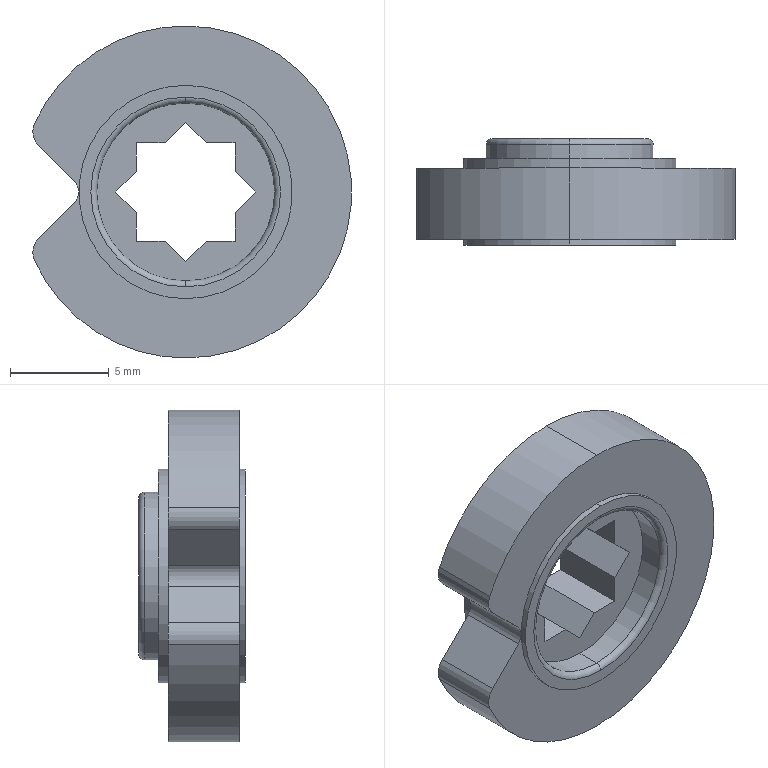Part | STEP file | PCS-04A-3_1_2.stp | 1 solid | 42 faces | box 16.138 x 5.4 x 16.8 mm | volume 681.99 mm3 | plane 24 | cylinder 14 | torus 4 | commonest cylinder face diameters 10.8 x4 16.8 x3 2 x2 8.5 x2 9 x2 1.568 x1
STEP:
#1=CARTESIAN_POINT('',(0.,5.1,3.95));
#2=VERTEX_POINT('',#1);
#3=CARTESIAN_POINT('',(0.,4.8,4.25));
#4=VERTEX_POINT('',#3);
#5=CARTESIAN_POINT('',(0.,4.8,3.95));
#6=DIRECTION('',(1.,0.,0.));
#7=DIRECTION('',(0.,1.,0.));
#8=AXIS2_PLACEMENT_3D('',#5,#6,#7);
#9=CIRCLE('',#8,0.3);
#10=EDGE_CURVE('',#2,#4,#9,.T.);
#11=ORIENTED_EDGE('',*,*,#10,.T.);
#12=CARTESIAN_POINT('',(0.,4.8,-4.25));
#13=VERTEX_POINT('',#12);
#14=CARTESIAN_POINT('',(0.,4.8,0.));
#15=DIRECTION('',(0.,-1.,0.));
#16=DIRECTION('',(0.,0.,-1.));
#17=AXIS2_PLACEMENT_3D('',#14,#15,#16);
#18=CIRCLE('',#17,4.25);
#19=EDGE_CURVE('',#13,#4,#18,.T.);
#20=ORIENTED_EDGE('',*,*,#19,.F.);
#21=CARTESIAN_POINT('',(0.,5.1,-3.95));
#22=VERTEX_POINT('',#21);
#23=CARTESIAN_POINT('',(0.,4.8,-3.95));
#24=DIRECTION('',(1.,0.,0.));
#25=DIRECTION('',(0.,0.,-1.));
#26=AXIS2_PLACEMENT_3D('',#23,#24,#25);
#27=CIRCLE('',#26,0.3);
#28=EDGE_CURVE('',#13,#22,#27,.T.);
#29=ORIENTED_EDGE('',*,*,#28,.T.);
#30=CARTESIAN_POINT('',(0.,5.1,0.));
#31=DIRECTION('',(0.,-1.,0.));
#32=DIRECTION('',(0.,0.,-1.));
#33=AXIS2_PLACEMENT_3D('',#30,#31,#32);
#34=CIRCLE('',#33,3.95);
#35=EDGE_CURVE('',#22,#2,#34,.T.);
#36=ORIENTED_EDGE('',*,*,#35,.T.);
#37=EDGE_LOOP('',(#11,#20,#29,#36));
#38=FACE_OUTER_BOUND('',#37,.T.);
#39=CARTESIAN_POINT('',(0.,4.8,0.));
#40=DIRECTION('',(0.,-1.,0.));
#41=DIRECTION('',(0.,0.,-1.));
#42=AXIS2_PLACEMENT_3D('',#39,#40,#41);
#43=TOROIDAL_SURFACE('',#42,3.95,0.3);
#44=ADVANCED_FACE('',(#38),#43,.T.);
#45=ORIENTED_EDGE('',*,*,#35,.F.);
#46=CARTESIAN_POINT('',(0.,5.1,0.));
#47=DIRECTION('',(0.,-1.,0.));
#48=DIRECTION('',(0.,0.,1.));
#49=AXIS2_PLACEMENT_3D('',#46,#47,#48);
#50=CIRCLE('',#49,3.95);
#51=EDGE_CURVE('',#2,#22,#50,.T.);
#52=ORIENTED_EDGE('',*,*,#51,.F.);
#53=EDGE_LOOP('',(#45,#52));
#54=FACE_OUTER_BOUND('',#53,.T.);
#55=CARTESIAN_POINT('',(-2.5,5.1,-2.5));
#56=VERTEX_POINT('',#55);
#57=CARTESIAN_POINT('',(-2.5,5.1,-1.036));
#58=VERTEX_POINT('',#57);
#59=CARTESIAN_POINT('',(-2.5,5.1,-2.5));
#60=DIRECTION('',(0.,0.,1.));
#61=VECTOR('',#60,1000.);
#62=LINE('',#59,#61);
#63=EDGE_CURVE('',#56,#58,#62,.T.);
#64=ORIENTED_EDGE('',*,*,#63,.F.);
#65=CARTESIAN_POINT('',(-1.036,5.1,-2.5));
#66=VERTEX_POINT('',#65);
#67=CARTESIAN_POINT('',(-1.036,5.1,-2.5));
#68=DIRECTION('',(-1.,0.,0.));
#69=VECTOR('',#68,1000.);
#70=LINE('',#67,#69);
#71=EDGE_CURVE('',#66,#56,#70,.T.);
#72=ORIENTED_EDGE('',*,*,#71,.F.);
#73=CARTESIAN_POINT('',(0.,5.1,-3.536));
#74=VERTEX_POINT('',#73);
#75=CARTESIAN_POINT('',(0.,5.1,-3.536));
#76=DIRECTION('',(-0.7071,0.,0.7071));
#77=VECTOR('',#76,1000.);
#78=LINE('',#75,#77);
#79=EDGE_CURVE('',#74,#66,#78,.T.);
#80=ORIENTED_EDGE('',*,*,#79,.F.);
#81=CARTESIAN_POINT('',(1.036,5.1,-2.5));
#82=VERTEX_POINT('',#81);
#83=CARTESIAN_POINT('',(0.,5.1,-3.536));
#84=DIRECTION('',(0.7071,0.,0.7071));
#85=VECTOR('',#84,1000.);
#86=LINE('',#83,#85);
#87=EDGE_CURVE('',#74,#82,#86,.T.);
#88=ORIENTED_EDGE('',*,*,#87,.T.);
#89=CARTESIAN_POINT('',(2.5,5.1,-2.5));
#90=VERTEX_POINT('',#89);
#91=CARTESIAN_POINT('',(2.5,5.1,-2.5));
#92=DIRECTION('',(-1.,0.,0.));
#93=VECTOR('',#92,1000.);
#94=LINE('',#91,#93);
#95=EDGE_CURVE('',#90,#82,#94,.T.);
#96=ORIENTED_EDGE('',*,*,#95,.F.);
#97=CARTESIAN_POINT('',(2.5,5.1,-1.036));
#98=VERTEX_POINT('',#97);
#99=CARTESIAN_POINT('',(2.5,5.1,-1.036));
#100=DIRECTION('',(0.,0.,-1.));
#101=VECTOR('',#100,1000.);
#102=LINE('',#99,#101);
#103=EDGE_CURVE('',#98,#90,#102,.T.);
#104=ORIENTED_EDGE('',*,*,#103,.F.);
#105=CARTESIAN_POINT('',(3.536,5.1,0.));
#106=VERTEX_POINT('',#105);
#107=CARTESIAN_POINT('',(2.5,5.1,-1.036));
#108=DIRECTION('',(0.7071,0.,0.7071));
#109=VECTOR('',#108,1000.);
#110=LINE('',#107,#109);
#111=EDGE_CURVE('',#98,#106,#110,.T.);
#112=ORIENTED_EDGE('',*,*,#111,.T.);
#113=CARTESIAN_POINT('',(2.5,5.1,1.036));
#114=VERTEX_POINT('',#113);
#115=CARTESIAN_POINT('',(2.5,5.1,1.036));
#116=DIRECTION('',(0.7071,0.,-0.7071));
#117=VECTOR('',#116,1000.);
#118=LINE('',#115,#117);
#119=EDGE_CURVE('',#114,#106,#118,.T.);
#120=ORIENTED_EDGE('',*,*,#119,.F.);
#121=CARTESIAN_POINT('',(2.5,5.1,2.5));
#122=VERTEX_POINT('',#121);
#123=CARTESIAN_POINT('',(2.5,5.1,2.5));
#124=DIRECTION('',(0.,0.,-1.));
#125=VECTOR('',#124,1000.);
#126=LINE('',#123,#125);
#127=EDGE_CURVE('',#122,#114,#126,.T.);
#128=ORIENTED_EDGE('',*,*,#127,.F.);
#129=CARTESIAN_POINT('',(1.036,5.1,2.5));
#130=VERTEX_POINT('',#129);
#131=CARTESIAN_POINT('',(1.036,5.1,2.5));
#132=DIRECTION('',(1.,0.,0.));
#133=VECTOR('',#132,1000.);
#134=LINE('',#131,#133);
#135=EDGE_CURVE('',#130,#122,#134,.T.);
#136=ORIENTED_EDGE('',*,*,#135,.F.);
#137=CARTESIAN_POINT('',(0.,5.1,3.536));
#138=VERTEX_POINT('',#137);
#139=CARTESIAN_POINT('',(0.,5.1,3.536));
#140=DIRECTION('',(0.7071,0.,-0.7071));
#141=VECTOR('',#140,1000.);
#142=LINE('',#139,#141);
#143=EDGE_CURVE('',#138,#130,#142,.T.);
#144=ORIENTED_EDGE('',*,*,#143,.F.);
#145=CARTESIAN_POINT('',(-1.036,5.1,2.5));
#146=VERTEX_POINT('',#145);
#147=CARTESIAN_POINT('',(0.,5.1,3.536));
#148=DIRECTION('',(-0.7071,0.,-0.7071));
#149=VECTOR('',#148,1000.);
#150=LINE('',#147,#149);
#151=EDGE_CURVE('',#138,#146,#150,.T.);
#152=ORIENTED_EDGE('',*,*,#151,.T.);
#153=CARTESIAN_POINT('',(-2.5,5.1,2.5));
#154=VERTEX_POINT('',#153);
#155=CARTESIAN_POINT('',(-2.5,5.1,2.5));
#156=DIRECTION('',(1.,0.,0.));
#157=VECTOR('',#156,1000.);
#158=LINE('',#155,#157);
#159=EDGE_CURVE('',#154,#146,#158,.T.);
#160=ORIENTED_EDGE('',*,*,#159,.F.);
#161=CARTESIAN_POINT('',(-2.5,5.1,1.036));
#162=VERTEX_POINT('',#161);
#163=CARTESIAN_POINT('',(-2.5,5.1,1.036));
#164=DIRECTION('',(0.,0.,1.));
#165=VECTOR('',#164,1000.);
#166=LINE('',#163,#165);
#167=EDGE_CURVE('',#162,#154,#166,.T.);
#168=ORIENTED_EDGE('',*,*,#167,.F.);
#169=CARTESIAN_POINT('',(-3.536,5.1,0.));
#170=VERTEX_POINT('',#169);
#171=CARTESIAN_POINT('',(-2.5,5.1,1.036));
#172=DIRECTION('',(-0.7071,0.,-0.7071));
#173=VECTOR('',#172,1000.);
#174=LINE('',#171,#173);
#175=EDGE_CURVE('',#162,#170,#174,.T.);
#176=ORIENTED_EDGE('',*,*,#175,.T.);
#177=CARTESIAN_POINT('',(-2.5,5.1,-1.036));
#178=DIRECTION('',(-0.7071,0.,0.7071));
#179=VECTOR('',#178,1000.);
#180=LINE('',#177,#179);
#181=EDGE_CURVE('',#58,#170,#180,.T.);
#182=ORIENTED_EDGE('',*,*,#181,.F.);
#183=EDGE_LOOP('',(#64,#72,#80,#88,#96,#104,#112,#120,#128,#136,#144,#152,#160,#168,#176,#182));
#184=FACE_BOUND('',#183,.T.);
#185=CARTESIAN_POINT('',(0.,5.1,0.));
#186=DIRECTION('',(0.,-1.,0.));
#187=DIRECTION('',(0.,0.,-1.));
#188=AXIS2_PLACEMENT_3D('',#185,#186,#187);
#189=PLANE('',#188);
#190=ADVANCED_FACE('',(#54,#184),#189,.F.);
#191=ORIENTED_EDGE('',*,*,#51,.T.);
#192=ORIENTED_EDGE('',*,*,#28,.F.);
#193=CARTESIAN_POINT('',(0.,4.8,0.));
#194=DIRECTION('',(0.,-1.,0.));
#195=DIRECTION('',(0.,0.,1.));
#196=AXIS2_PLACEMENT_3D('',#193,#194,#195);
#197=CIRCLE('',#196,4.25);
#198=EDGE_CURVE('',#4,#13,#197,.T.);
#199=ORIENTED_EDGE('',*,*,#198,.F.);
#200=ORIENTED_EDGE('',*,*,#10,.F.);
#201=EDGE_LOOP('',(#191,#192,#199,#200));
#202=FACE_OUTER_BOUND('',#201,.T.);
#203=CARTESIAN_POINT('',(0.,4.8,0.));
#204=DIRECTION('',(0.,-1.,0.));
#205=DIRECTION('',(0.,0.,-1.));
#206=AXIS2_PLACEMENT_3D('',#203,#204,#205);
#207=TOROIDAL_SURFACE('',#206,3.95,0.3);
#208=ADVANCED_FACE('',(#202),#207,.T.);
#209=ORIENTED_EDGE('',*,*,#198,.T.);
#210=CARTESIAN_POINT('',(0.,4.1,-4.25));
#211=VERTEX_POINT('',#210);
#212=CARTESIAN_POINT('',(0.,4.1,-4.25));
#213=DIRECTION('',(0.,1.,0.));
#214=VECTOR('',#213,1000.);
#215=LINE('',#212,#214);
#216=EDGE_CURVE('',#211,#13,#215,.T.);
#217=ORIENTED_EDGE('',*,*,#216,.F.);
#218=CARTESIAN_POINT('',(0.,4.1,4.25));
#219=VERTEX_POINT('',#218);
#220=CARTESIAN_POINT('',(0.,4.1,0.));
#221=DIRECTION('',(0.,1.,0.));
#222=DIRECTION('',(0.,0.,-1.));
#223=AXIS2_PLACEMENT_3D('',#220,#221,#222);
#224=CIRCLE('',#223,4.25);
#225=EDGE_CURVE('',#211,#219,#224,.T.);
#226=ORIENTED_EDGE('',*,*,#225,.T.);
#227=CARTESIAN_POINT('',(0.,4.8,4.25));
#228=DIRECTION('',(0.,-1.,0.));
#229=VECTOR('',#228,1000.);
#230=LINE('',#227,#229);
#231=EDGE_CURVE('',#4,#219,#230,.T.);
#232=ORIENTED_EDGE('',*,*,#231,.F.);
#233=EDGE_LOOP('',(#209,#217,#226,#232));
#234=FACE_OUTER_BOUND('',#233,.T.);
#235=CARTESIAN_POINT('',(0.,4.1,0.));
#236=DIRECTION('',(0.,-1.,0.));
#237=DIRECTION('',(0.,0.,-1.));
#238=AXIS2_PLACEMENT_3D('',#235,#236,#237);
#239=CYLINDRICAL_SURFACE('',#238,4.25);
#240=ADVANCED_FACE('',(#234),#239,.T.);
#241=ORIENTED_EDGE('',*,*,#231,.T.);
#242=CARTESIAN_POINT('',(0.,4.1,0.));
#243=DIRECTION('',(0.,1.,0.));
#244=DIRECTION('',(0.,0.,1.));
#245=AXIS2_PLACEMENT_3D('',#242,#243,#244);
#246=CIRCLE('',#245,4.25);
#247=EDGE_CURVE('',#219,#211,#246,.T.);
#248=ORIENTED_EDGE('',*,*,#247,.T.);
#249=ORIENTED_EDGE('',*,*,#216,.T.);
#250=ORIENTED_EDGE('',*,*,#19,.T.);
#251=EDGE_LOOP('',(#241,#248,#249,#250));
#252=FACE_OUTER_BOUND('',#251,.T.);
#253=CARTESIAN_POINT('',(0.,4.1,0.));
#254=DIRECTION('',(0.,-1.,0.));
#255=DIRECTION('',(0.,0.,-1.));
#256=AXIS2_PLACEMENT_3D('',#253,#254,#255);
#257=CYLINDRICAL_SURFACE('',#256,4.25);
#258=ADVANCED_FACE('',(#252),#257,.T.);
#259=CARTESIAN_POINT('',(0.,4.1,-5.4));
#260=VERTEX_POINT('',#259);
#261=CARTESIAN_POINT('',(0.,4.1,5.4));
#262=VERTEX_POINT('',#261);
#263=CARTESIAN_POINT('',(0.,4.1,0.));
#264=DIRECTION('',(0.,-1.,0.));
#265=DIRECTION('',(0.,0.,-1.));
#266=AXIS2_PLACEMENT_3D('',#263,#264,#265);
#267=CIRCLE('',#266,5.4);
#268=EDGE_CURVE('',#260,#262,#267,.T.);
#269=ORIENTED_EDGE('',*,*,#268,.F.);
#270=CARTESIAN_POINT('',(0.,4.1,0.));
#271=DIRECTION('',(0.,-1.,0.));
#272=DIRECTION('',(0.,0.,1.));
#273=AXIS2_PLACEMENT_3D('',#270,#271,#272);
#274=CIRCLE('',#273,5.4);
#275=EDGE_CURVE('',#262,#260,#274,.T.);
#276=ORIENTED_EDGE('',*,*,#275,.F.);
#277=EDGE_LOOP('',(#269,#276));
#278=FACE_OUTER_BOUND('',#277,.T.);
#279=ORIENTED_EDGE('',*,*,#247,.F.);
#280=ORIENTED_EDGE('',*,*,#225,.F.);
#281=EDGE_LOOP('',(#279,#280));
#282=FACE_BOUND('',#281,.T.);
#283=CARTESIAN_POINT('',(0.,4.1,0.));
#284=DIRECTION('',(0.,1.,0.));
#285=DIRECTION('',(1.,0.,0.));
#286=AXIS2_PLACEMENT_3D('',#283,#284,#285);
#287=PLANE('',#286);
#288=ADVANCED_FACE('',(#278,#282),#287,.T.);
#289=ORIENTED_EDGE('',*,*,#275,.T.);
#290=CARTESIAN_POINT('',(0.,3.6,-5.4));
#291=VERTEX_POINT('',#290);
#292=CARTESIAN_POINT('',(0.,3.6,-5.4));
#293=DIRECTION('',(0.,1.,0.));
#294=VECTOR('',#293,1000.);
#295=LINE('',#292,#294);
#296=EDGE_CURVE('',#291,#260,#295,.T.);
#297=ORIENTED_EDGE('',*,*,#296,.F.);
#298=CARTESIAN_POINT('',(0.,3.6,5.4));
#299=VERTEX_POINT('',#298);
#300=CARTESIAN_POINT('',(0.,3.6,0.));
#301=DIRECTION('',(0.,1.,0.));
#302=DIRECTION('',(0.,0.,-1.));
#303=AXIS2_PLACEMENT_3D('',#300,#301,#302);
#304=CIRCLE('',#303,5.4);
#305=EDGE_CURVE('',#291,#299,#304,.T.);
#306=ORIENTED_EDGE('',*,*,#305,.T.);
#307=CARTESIAN_POINT('',(0.,4.1,5.4));
#308=DIRECTION('',(0.,-1.,0.));
#309=VECTOR('',#308,1000.);
#310=LINE('',#307,#309);
#311=EDGE_CURVE('',#262,#299,#310,.T.);
#312=ORIENTED_EDGE('',*,*,#311,.F.);
#313=EDGE_LOOP('',(#289,#297,#306,#312));
#314=FACE_OUTER_BOUND('',#313,.T.);
#315=CARTESIAN_POINT('',(0.,3.6,0.));
#316=DIRECTION('',(0.,-1.,0.));
#317=DIRECTION('',(0.,0.,-1.));
#318=AXIS2_PLACEMENT_3D('',#315,#316,#317);
#319=CYLINDRICAL_SURFACE('',#318,5.4);
#320=ADVANCED_FACE('',(#314),#319,.T.);
#321=ORIENTED_EDGE('',*,*,#311,.T.);
#322=CARTESIAN_POINT('',(0.,3.6,0.));
#323=DIRECTION('',(0.,1.,0.));
#324=DIRECTION('',(0.,0.,1.));
#325=AXIS2_PLACEMENT_3D('',#322,#323,#324);
#326=CIRCLE('',#325,5.4);
#327=EDGE_CURVE('',#299,#291,#326,.T.);
#328=ORIENTED_EDGE('',*,*,#327,.T.);
#329=ORIENTED_EDGE('',*,*,#296,.T.);
#330=ORIENTED_EDGE('',*,*,#268,.T.);
#331=EDGE_LOOP('',(#321,#328,#329,#330));
#332=FACE_OUTER_BOUND('',#331,.T.);
#333=CARTESIAN_POINT('',(0.,3.6,0.));
#334=DIRECTION('',(0.,-1.,0.));
#335=DIRECTION('',(0.,0.,-1.));
#336=AXIS2_PLACEMENT_3D('',#333,#334,#335);
#337=CYLINDRICAL_SURFACE('',#336,5.4);
#338=ADVANCED_FACE('',(#332),#337,.T.);
#339=CARTESIAN_POINT('',(0.,3.6,-8.4));
#340=VERTEX_POINT('',#339);
#341=CARTESIAN_POINT('',(0.,3.6,8.4));
#342=VERTEX_POINT('',#341);
#343=CARTESIAN_POINT('',(0.,3.6,0.));
#344=DIRECTION('',(0.,-1.,0.));
#345=DIRECTION('',(0.,0.,-1.));
#346=AXIS2_PLACEMENT_3D('',#343,#344,#345);
#347=CIRCLE('',#346,8.4);
#348=EDGE_CURVE('',#340,#342,#347,.T.);
#349=ORIENTED_EDGE('',*,*,#348,.F.);
#350=CARTESIAN_POINT('',(-7.649,3.6,-3.472));
#351=VERTEX_POINT('',#350);
#352=CARTESIAN_POINT('',(0.,3.6,0.));
#353=DIRECTION('',(0.,-1.,0.));
#354=DIRECTION('',(-0.9106,0.,-0.4133));
#355=AXIS2_PLACEMENT_3D('',#352,#353,#354);
#356=CIRCLE('',#355,8.4);
#357=EDGE_CURVE('',#351,#340,#356,.T.);
#358=ORIENTED_EDGE('',*,*,#357,.F.);
#359=CARTESIAN_POINT('',(-7.446,3.6,-2.351));
#360=VERTEX_POINT('',#359);
#361=CARTESIAN_POINT('',(-6.738,3.6,-3.058));
#362=DIRECTION('',(0.,-1.,0.));
#363=DIRECTION('',(-0.7071,0.,0.7071));
#364=AXIS2_PLACEMENT_3D('',#361,#362,#363);
#365=CIRCLE('',#364,1.);
#366=EDGE_CURVE('',#360,#351,#365,.T.);
#367=ORIENTED_EDGE('',*,*,#366,.F.);
#368=CARTESIAN_POINT('',(-5.607,3.6,-0.5127));
#369=VERTEX_POINT('',#368);
#370=CARTESIAN_POINT('',(-7.446,3.6,-2.351));
#371=DIRECTION('',(0.7071,0.,0.7071));
#372=VECTOR('',#371,1000.);
#373=LINE('',#370,#372);
#374=EDGE_CURVE('',#360,#369,#373,.T.);
#375=ORIENTED_EDGE('',*,*,#374,.T.);
#376=CARTESIAN_POINT('',(-5.607,3.6,0.5127));
#377=VERTEX_POINT('',#376);
#378=CARTESIAN_POINT('',(-6.2,3.6,0.));
#379=DIRECTION('',(0.,1.,0.));
#380=DIRECTION('',(0.7564,0.,0.6541));
#381=AXIS2_PLACEMENT_3D('',#378,#379,#380);
#382=CIRCLE('',#381,0.7838);
#383=EDGE_CURVE('',#377,#369,#382,.T.);
#384=ORIENTED_EDGE('',*,*,#383,.F.);
#385=CARTESIAN_POINT('',(-7.446,3.6,2.351));
#386=VERTEX_POINT('',#385);
#387=CARTESIAN_POINT('',(-5.607,3.6,0.5127));
#388=DIRECTION('',(-0.7071,0.,0.7071));
#389=VECTOR('',#388,1000.);
#390=LINE('',#387,#389);
#391=EDGE_CURVE('',#377,#386,#390,.T.);
#392=ORIENTED_EDGE('',*,*,#391,.T.);
#393=CARTESIAN_POINT('',(-7.649,3.6,3.472));
#394=VERTEX_POINT('',#393);
#395=CARTESIAN_POINT('',(-6.738,3.6,3.058));
#396=DIRECTION('',(0.,-1.,0.));
#397=DIRECTION('',(-0.9106,0.,0.4133));
#398=AXIS2_PLACEMENT_3D('',#395,#396,#397);
#399=CIRCLE('',#398,1.);
#400=EDGE_CURVE('',#394,#386,#399,.T.);
#401=ORIENTED_EDGE('',*,*,#400,.F.);
#402=CARTESIAN_POINT('',(0.,3.6,0.));
#403=DIRECTION('',(0.,-1.,0.));
#404=DIRECTION('',(0.,0.,1.));
#405=AXIS2_PLACEMENT_3D('',#402,#403,#404);
#406=CIRCLE('',#405,8.4);
#407=EDGE_CURVE('',#342,#394,#406,.T.);
#408=ORIENTED_EDGE('',*,*,#407,.F.);
#409=EDGE_LOOP('',(#349,#358,#367,#375,#384,#392,#401,#408));
#410=FACE_OUTER_BOUND('',#409,.T.);
#411=ORIENTED_EDGE('',*,*,#327,.F.);
#412=ORIENTED_EDGE('',*,*,#305,.F.);
#413=EDGE_LOOP('',(#411,#412));
#414=FACE_BOUND('',#413,.T.);
#415=CARTESIAN_POINT('',(0.,3.6,0.));
#416=DIRECTION('',(0.,1.,0.));
#417=DIRECTION('',(1.,0.,0.));
#418=AXIS2_PLACEMENT_3D('',#415,#416,#417);
#419=PLANE('',#418);
#420=ADVANCED_FACE('',(#410,#414),#419,.T.);
#421=ORIENTED_EDGE('',*,*,#407,.T.);
#422=CARTESIAN_POINT('',(-7.649,0.,3.472));
#423=VERTEX_POINT('',#422);
#424=CARTESIAN_POINT('',(-7.649,3.6,3.472));
#425=DIRECTION('',(0.,-1.,0.));
#426=VECTOR('',#425,1000.);
#427=LINE('',#424,#426);
#428=EDGE_CURVE('',#394,#423,#427,.T.);
#429=ORIENTED_EDGE('',*,*,#428,.T.);
#430=CARTESIAN_POINT('',(0.,0.,8.4));
#431=VERTEX_POINT('',#430);
#432=CARTESIAN_POINT('',(0.,0.,0.));
#433=DIRECTION('',(0.,1.,0.));
#434=DIRECTION('',(-0.9106,0.,0.4133));
#435=AXIS2_PLACEMENT_3D('',#432,#433,#434);
#436=CIRCLE('',#435,8.4);
#437=EDGE_CURVE('',#423,#431,#436,.T.);
#438=ORIENTED_EDGE('',*,*,#437,.T.);
#439=CARTESIAN_POINT('',(0.,3.6,8.4));
#440=DIRECTION('',(0.,-1.,0.));
#441=VECTOR('',#440,1000.);
#442=LINE('',#439,#441);
#443=EDGE_CURVE('',#342,#431,#442,.T.);
#444=ORIENTED_EDGE('',*,*,#443,.F.);
#445=EDGE_LOOP('',(#421,#429,#438,#444));
#446=FACE_OUTER_BOUND('',#445,.T.);
#447=CARTESIAN_POINT('',(0.,0.,0.));
#448=DIRECTION('',(0.,-1.,0.));
#449=DIRECTION('',(0.,0.,-1.));
#450=AXIS2_PLACEMENT_3D('',#447,#448,#449);
#451=CYLINDRICAL_SURFACE('',#450,8.4);
#452=ADVANCED_FACE('',(#446),#451,.T.);
#453=ORIENTED_EDGE('',*,*,#443,.T.);
#454=CARTESIAN_POINT('',(0.,0.,-8.4));
#455=VERTEX_POINT('',#454);
#456=CARTESIAN_POINT('',(0.,0.,0.));
#457=DIRECTION('',(0.,1.,0.));
#458=DIRECTION('',(0.,0.,1.));
#459=AXIS2_PLACEMENT_3D('',#456,#457,#458);
#460=CIRCLE('',#459,8.4);
#461=EDGE_CURVE('',#431,#455,#460,.T.);
#462=ORIENTED_EDGE('',*,*,#461,.T.);
#463=CARTESIAN_POINT('',(0.,0.,-8.4));
#464=DIRECTION('',(0.,1.,0.));
#465=VECTOR('',#464,1000.);
#466=LINE('',#463,#465);
#467=EDGE_CURVE('',#455,#340,#466,.T.);
#468=ORIENTED_EDGE('',*,*,#467,.T.);
#469=ORIENTED_EDGE('',*,*,#348,.T.);
#470=EDGE_LOOP('',(#453,#462,#468,#469));
#471=FACE_OUTER_BOUND('',#470,.T.);
#472=CARTESIAN_POINT('',(0.,0.,0.));
#473=DIRECTION('',(0.,-1.,0.));
#474=DIRECTION('',(0.,0.,-1.));
#475=AXIS2_PLACEMENT_3D('',#472,#473,#474);
#476=CYLINDRICAL_SURFACE('',#475,8.4);
#477=ADVANCED_FACE('',(#471),#476,.T.);
#478=ORIENTED_EDGE('',*,*,#467,.F.);
#479=CARTESIAN_POINT('',(-7.649,0.,-3.472));
#480=VERTEX_POINT('',#479);
#481=CARTESIAN_POINT('',(0.,0.,0.));
#482=DIRECTION('',(0.,1.,0.));
#483=DIRECTION('',(0.,0.,-1.));
#484=AXIS2_PLACEMENT_3D('',#481,#482,#483);
#485=CIRCLE('',#484,8.4);
#486=EDGE_CURVE('',#455,#480,#485,.T.);
#487=ORIENTED_EDGE('',*,*,#486,.T.);
#488=CARTESIAN_POINT('',(-7.649,0.,-3.472));
#489=DIRECTION('',(0.,1.,0.));
#490=VECTOR('',#489,1000.);
#491=LINE('',#488,#490);
#492=EDGE_CURVE('',#480,#351,#491,.T.);
#493=ORIENTED_EDGE('',*,*,#492,.T.);
#494=ORIENTED_EDGE('',*,*,#357,.T.);
#495=EDGE_LOOP('',(#478,#487,#493,#494));
#496=FACE_OUTER_BOUND('',#495,.T.);
#497=CARTESIAN_POINT('',(0.,0.,0.));
#498=DIRECTION('',(0.,-1.,0.));
#499=DIRECTION('',(0.,0.,-1.));
#500=AXIS2_PLACEMENT_3D('',#497,#498,#499);
#501=CYLINDRICAL_SURFACE('',#500,8.4);
#502=ADVANCED_FACE('',(#496),#501,.T.);
#503=ORIENTED_EDGE('',*,*,#492,.F.);
#504=CARTESIAN_POINT('',(-7.446,0.,-2.351));
#505=VERTEX_POINT('',#504);
#506=CARTESIAN_POINT('',(-6.738,0.,-3.058));
#507=DIRECTION('',(0.,1.,0.));
#508=DIRECTION('',(-0.9106,0.,-0.4133));
#509=AXIS2_PLACEMENT_3D('',#506,#507,#508);
#510=CIRCLE('',#509,1.);
#511=EDGE_CURVE('',#480,#505,#510,.T.);
#512=ORIENTED_EDGE('',*,*,#511,.T.);
#513=CARTESIAN_POINT('',(-7.446,0.,-2.351));
#514=DIRECTION('',(0.,1.,0.));
#515=VECTOR('',#514,1000.);
#516=LINE('',#513,#515);
#517=EDGE_CURVE('',#505,#360,#516,.T.);
#518=ORIENTED_EDGE('',*,*,#517,.T.);
#519=ORIENTED_EDGE('',*,*,#366,.T.);
#520=EDGE_LOOP('',(#503,#512,#518,#519));
#521=FACE_OUTER_BOUND('',#520,.T.);
#522=CARTESIAN_POINT('',(-6.738,3.6,-3.058));
#523=DIRECTION('',(0.,1.,0.));
#524=DIRECTION('',(0.,0.,1.));
#525=AXIS2_PLACEMENT_3D('',#522,#523,#524);
#526=CYLINDRICAL_SURFACE('',#525,1.);
#527=ADVANCED_FACE('',(#521),#526,.T.);
#528=ORIENTED_EDGE('',*,*,#517,.F.);
#529=CARTESIAN_POINT('',(-5.607,0.,-0.5127));
#530=VERTEX_POINT('',#529);
#531=CARTESIAN_POINT('',(-5.607,0.,-0.5127));
#532=DIRECTION('',(-0.7071,0.,-0.7071));
#533=VECTOR('',#532,1000.);
#534=LINE('',#531,#533);
#535=EDGE_CURVE('',#530,#505,#534,.T.);
#536=ORIENTED_EDGE('',*,*,#535,.F.);
#537=CARTESIAN_POINT('',(-5.607,3.6,-0.5127));
#538=DIRECTION('',(0.,-1.,0.));
#539=VECTOR('',#538,1000.);
#540=LINE('',#537,#539);
#541=EDGE_CURVE('',#369,#530,#540,.T.);
#542=ORIENTED_EDGE('',*,*,#541,.F.);
#543=ORIENTED_EDGE('',*,*,#374,.F.);
#544=EDGE_LOOP('',(#528,#536,#542,#543));
#545=FACE_OUTER_BOUND('',#544,.T.);
#546=CARTESIAN_POINT('',(-11.858,0.,-6.764));
#547=DIRECTION('',(0.7071,0.,-0.7071));
#548=DIRECTION('',(0.,-1.,0.));
#549=AXIS2_PLACEMENT_3D('',#546,#547,#548);
#550=PLANE('',#549);
#551=ADVANCED_FACE('',(#545),#550,.F.);
#552=ORIENTED_EDGE('',*,*,#541,.T.);
#553=CARTESIAN_POINT('',(-5.607,0.,0.5127));
#554=VERTEX_POINT('',#553);
#555=CARTESIAN_POINT('',(-6.2,0.,0.));
#556=DIRECTION('',(0.,-1.,0.));
#557=DIRECTION('',(0.7564,0.,-0.6541));
#558=AXIS2_PLACEMENT_3D('',#555,#556,#557);
#559=CIRCLE('',#558,0.7838);
#560=EDGE_CURVE('',#530,#554,#559,.T.);
#561=ORIENTED_EDGE('',*,*,#560,.T.);
#562=CARTESIAN_POINT('',(-5.607,3.6,0.5127));
#563=DIRECTION('',(0.,-1.,0.));
#564=VECTOR('',#563,1000.);
#565=LINE('',#562,#564);
#566=EDGE_CURVE('',#377,#554,#565,.T.);
#567=ORIENTED_EDGE('',*,*,#566,.F.);
#568=ORIENTED_EDGE('',*,*,#383,.T.);
#569=EDGE_LOOP('',(#552,#561,#567,#568));
#570=FACE_OUTER_BOUND('',#569,.T.);
#571=CARTESIAN_POINT('',(-6.2,0.,0.));
#572=DIRECTION('',(0.,1.,0.));
#573=DIRECTION('',(0.,0.,1.));
#574=AXIS2_PLACEMENT_3D('',#571,#572,#573);
#575=CYLINDRICAL_SURFACE('',#574,0.7838);
#576=ADVANCED_FACE('',(#570),#575,.F.);
#577=ORIENTED_EDGE('',*,*,#566,.T.);
#578=CARTESIAN_POINT('',(-7.446,0.,2.351));
#579=VERTEX_POINT('',#578);
#580=CARTESIAN_POINT('',(-7.446,0.,2.351));
#581=DIRECTION('',(0.7071,0.,-0.7071));
#582=VECTOR('',#581,1000.);
#583=LINE('',#580,#582);
#584=EDGE_CURVE('',#579,#554,#583,.T.);
#585=ORIENTED_EDGE('',*,*,#584,.F.);
#586=CARTESIAN_POINT('',(-7.446,0.,2.351));
#587=DIRECTION('',(0.,1.,0.));
#588=VECTOR('',#587,1000.);
#589=LINE('',#586,#588);
#590=EDGE_CURVE('',#579,#386,#589,.T.);
#591=ORIENTED_EDGE('',*,*,#590,.T.);
#592=ORIENTED_EDGE('',*,*,#391,.F.);
#593=EDGE_LOOP('',(#577,#585,#591,#592));
#594=FACE_OUTER_BOUND('',#593,.T.);
#595=CARTESIAN_POINT('',(-11.858,0.,6.764));
#596=DIRECTION('',(-0.7071,0.,-0.7071));
#597=DIRECTION('',(-0.7071,0.,0.7071));
#598=AXIS2_PLACEMENT_3D('',#595,#596,#597);
#599=PLANE('',#598);
#600=ADVANCED_FACE('',(#594),#599,.T.);
#601=ORIENTED_EDGE('',*,*,#590,.F.);
#602=CARTESIAN_POINT('',(-6.738,0.,3.058));
#603=DIRECTION('',(0.,1.,0.));
#604=DIRECTION('',(-0.7071,0.,-0.7071));
#605=AXIS2_PLACEMENT_3D('',#602,#603,#604);
#606=CIRCLE('',#605,1.);
#607=EDGE_CURVE('',#579,#423,#606,.T.);
#608=ORIENTED_EDGE('',*,*,#607,.T.);
#609=ORIENTED_EDGE('',*,*,#428,.F.);
#610=ORIENTED_EDGE('',*,*,#400,.T.);
#611=EDGE_LOOP('',(#601,#608,#609,#610));
#612=FACE_OUTER_BOUND('',#611,.T.);
#613=CARTESIAN_POINT('',(-6.738,3.6,3.058));
#614=DIRECTION('',(0.,1.,0.));
#615=DIRECTION('',(0.,0.,1.));
#616=AXIS2_PLACEMENT_3D('',#613,#614,#615);
#617=CYLINDRICAL_SURFACE('',#616,1.);
#618=ADVANCED_FACE('',(#612),#617,.T.);
#619=ORIENTED_EDGE('',*,*,#486,.F.);
#620=ORIENTED_EDGE('',*,*,#461,.F.);
#621=ORIENTED_EDGE('',*,*,#437,.F.);
#622=ORIENTED_EDGE('',*,*,#607,.F.);
#623=ORIENTED_EDGE('',*,*,#584,.T.);
#624=ORIENTED_EDGE('',*,*,#560,.F.);
#625=ORIENTED_EDGE('',*,*,#535,.T.);
#626=ORIENTED_EDGE('',*,*,#511,.F.);
#627=EDGE_LOOP('',(#619,#620,#621,#622,#623,#624,#625,#626));
#628=FACE_OUTER_BOUND('',#627,.T.);
#629=CARTESIAN_POINT('',(0.,0.,5.4));
#630=VERTEX_POINT('',#629);
#631=CARTESIAN_POINT('',(0.,0.,-5.4));
#632=VERTEX_POINT('',#631);
#633=CARTESIAN_POINT('',(0.,0.,0.));
#634=DIRECTION('',(0.,-1.,0.));
#635=DIRECTION('',(0.,0.,1.));
#636=AXIS2_PLACEMENT_3D('',#633,#634,#635);
#637=CIRCLE('',#636,5.4);
#638=EDGE_CURVE('',#630,#632,#637,.T.);
#639=ORIENTED_EDGE('',*,*,#638,.F.);
#640=CARTESIAN_POINT('',(0.,0.,0.));
#641=DIRECTION('',(0.,-1.,0.));
#642=DIRECTION('',(0.,0.,-1.));
#643=AXIS2_PLACEMENT_3D('',#640,#641,#642);
#644=CIRCLE('',#643,5.4);
#645=EDGE_CURVE('',#632,#630,#644,.T.);
#646=ORIENTED_EDGE('',*,*,#645,.F.);
#647=EDGE_LOOP('',(#639,#646));
#648=FACE_BOUND('',#647,.T.);
#649=CARTESIAN_POINT('',(0.,0.,0.));
#650=DIRECTION('',(0.,1.,0.));
#651=DIRECTION('',(1.,0.,0.));
#652=AXIS2_PLACEMENT_3D('',#649,#650,#651);
#653=PLANE('',#652);
#654=ADVANCED_FACE('',(#628,#648),#653,.F.);
#655=CARTESIAN_POINT('',(0.,-0.3,-5.4));
#656=VERTEX_POINT('',#655);
#657=CARTESIAN_POINT('',(0.,-0.3,-5.4));
#658=DIRECTION('',(0.,1.,0.));
#659=VECTOR('',#658,1000.);
#660=LINE('',#657,#659);
#661=EDGE_CURVE('',#656,#632,#660,.T.);
#662=ORIENTED_EDGE('',*,*,#661,.T.);
#663=ORIENTED_EDGE('',*,*,#645,.T.);
#664=CARTESIAN_POINT('',(0.,-0.3,5.4));
#665=VERTEX_POINT('',#664);
#666=CARTESIAN_POINT('',(0.,0.,5.4));
#667=DIRECTION('',(0.,-1.,0.));
#668=VECTOR('',#667,1000.);
#669=LINE('',#666,#668);
#670=EDGE_CURVE('',#630,#665,#669,.T.);
#671=ORIENTED_EDGE('',*,*,#670,.T.);
#672=CARTESIAN_POINT('',(0.,-0.3,0.));
#673=DIRECTION('',(0.,1.,0.));
#674=DIRECTION('',(0.,0.,1.));
#675=AXIS2_PLACEMENT_3D('',#672,#673,#674);
#676=CIRCLE('',#675,5.4);
#677=EDGE_CURVE('',#665,#656,#676,.T.);
#678=ORIENTED_EDGE('',*,*,#677,.T.);
#679=EDGE_LOOP('',(#662,#663,#671,#678));
#680=FACE_OUTER_BOUND('',#679,.T.);
#681=CARTESIAN_POINT('',(0.,0.,0.));
#682=DIRECTION('',(0.,1.,0.));
#683=DIRECTION('',(0.,0.,1.));
#684=AXIS2_PLACEMENT_3D('',#681,#682,#683);
#685=CYLINDRICAL_SURFACE('',#684,5.4);
#686=ADVANCED_FACE('',(#680),#685,.T.);
#687=CARTESIAN_POINT('',(0.,-0.3,0.));
#688=DIRECTION('',(0.,1.,0.));
#689=DIRECTION('',(0.,0.,-1.));
#690=AXIS2_PLACEMENT_3D('',#687,#688,#689);
#691=CIRCLE('',#690,5.4);
#692=EDGE_CURVE('',#656,#665,#691,.T.);
#693=ORIENTED_EDGE('',*,*,#692,.F.);
#694=ORIENTED_EDGE('',*,*,#677,.F.);
#695=EDGE_LOOP('',(#693,#694));
#696=FACE_OUTER_BOUND('',#695,.T.);
#697=CARTESIAN_POINT('',(0.,-0.3,4.8));
#698=VERTEX_POINT('',#697);
#699=CARTESIAN_POINT('',(0.,-0.3,-4.8));
#700=VERTEX_POINT('',#699);
#701=CARTESIAN_POINT('',(0.,-0.3,0.));
#702=DIRECTION('',(0.,-1.,0.));
#703=DIRECTION('',(0.,0.,1.));
#704=AXIS2_PLACEMENT_3D('',#701,#702,#703);
#705=CIRCLE('',#704,4.8);
#706=EDGE_CURVE('',#698,#700,#705,.T.);
#707=ORIENTED_EDGE('',*,*,#706,.F.);
#708=CARTESIAN_POINT('',(0.,-0.3,0.));
#709=DIRECTION('',(0.,-1.,0.));
#710=DIRECTION('',(0.,0.,-1.));
#711=AXIS2_PLACEMENT_3D('',#708,#709,#710);
#712=CIRCLE('',#711,4.8);
#713=EDGE_CURVE('',#700,#698,#712,.T.);
#714=ORIENTED_EDGE('',*,*,#713,.F.);
#715=EDGE_LOOP('',(#707,#714));
#716=FACE_BOUND('',#715,.T.);
#717=CARTESIAN_POINT('',(0.,-0.3,0.));
#718=DIRECTION('',(0.,1.,0.));
#719=DIRECTION('',(1.,0.,0.));
#720=AXIS2_PLACEMENT_3D('',#717,#718,#719);
#721=PLANE('',#720);
#722=ADVANCED_FACE('',(#696,#716),#721,.F.);
#723=ORIENTED_EDGE('',*,*,#692,.T.);
#724=ORIENTED_EDGE('',*,*,#670,.F.);
#725=ORIENTED_EDGE('',*,*,#638,.T.);
#726=ORIENTED_EDGE('',*,*,#661,.F.);
#727=EDGE_LOOP('',(#723,#724,#725,#726));
#728=FACE_OUTER_BOUND('',#727,.T.);
#729=CARTESIAN_POINT('',(0.,0.,0.));
#730=DIRECTION('',(0.,1.,0.));
#731=DIRECTION('',(0.,0.,1.));
#732=AXIS2_PLACEMENT_3D('',#729,#730,#731);
#733=CYLINDRICAL_SURFACE('',#732,5.4);
#734=ADVANCED_FACE('',(#728),#733,.T.);
#735=CARTESIAN_POINT('',(0.,0.,-4.5));
#736=VERTEX_POINT('',#735);
#737=CARTESIAN_POINT('',(0.,0.,-4.8));
#738=DIRECTION('',(1.,0.,0.));
#739=DIRECTION('',(0.,0.,1.));
#740=AXIS2_PLACEMENT_3D('',#737,#738,#739);
#741=CIRCLE('',#740,0.3);
#742=EDGE_CURVE('',#736,#700,#741,.T.);
#743=ORIENTED_EDGE('',*,*,#742,.T.);
#744=ORIENTED_EDGE('',*,*,#713,.T.);
#745=CARTESIAN_POINT('',(0.,0.,4.5));
#746=VERTEX_POINT('',#745);
#747=CARTESIAN_POINT('',(0.,0.,4.8));
#748=DIRECTION('',(1.,0.,0.));
#749=DIRECTION('',(0.,-1.,0.));
#750=AXIS2_PLACEMENT_3D('',#747,#748,#749);
#751=CIRCLE('',#750,0.3);
#752=EDGE_CURVE('',#698,#746,#751,.T.);
#753=ORIENTED_EDGE('',*,*,#752,.T.);
#754=CARTESIAN_POINT('',(0.,0.,0.));
#755=DIRECTION('',(0.,-1.,0.));
#756=DIRECTION('',(0.,0.,-1.));
#757=AXIS2_PLACEMENT_3D('',#754,#755,#756);
#758=CIRCLE('',#757,4.5);
#759=EDGE_CURVE('',#736,#746,#758,.T.);
#760=ORIENTED_EDGE('',*,*,#759,.F.);
#761=EDGE_LOOP('',(#743,#744,#753,#760));
#762=FACE_OUTER_BOUND('',#761,.T.);
#763=CARTESIAN_POINT('',(0.,0.,0.));
#764=DIRECTION('',(0.,1.,0.));
#765=DIRECTION('',(0.,0.,1.));
#766=AXIS2_PLACEMENT_3D('',#763,#764,#765);
#767=TOROIDAL_SURFACE('',#766,4.8,0.3);
#768=ADVANCED_FACE('',(#762),#767,.T.);
#769=ORIENTED_EDGE('',*,*,#759,.T.);
#770=CARTESIAN_POINT('',(0.,1.2,4.5));
#771=VERTEX_POINT('',#770);
#772=CARTESIAN_POINT('',(0.,1.2,4.5));
#773=DIRECTION('',(0.,-1.,0.));
#774=VECTOR('',#773,1000.);
#775=LINE('',#772,#774);
#776=EDGE_CURVE('',#771,#746,#775,.T.);
#777=ORIENTED_EDGE('',*,*,#776,.F.);
#778=CARTESIAN_POINT('',(0.,1.2,-4.5));
#779=VERTEX_POINT('',#778);
#780=CARTESIAN_POINT('',(0.,1.2,0.));
#781=DIRECTION('',(0.,1.,0.));
#782=DIRECTION('',(0.,0.,1.));
#783=AXIS2_PLACEMENT_3D('',#780,#781,#782);
#784=CIRCLE('',#783,4.5);
#785=EDGE_CURVE('',#771,#779,#784,.T.);
#786=ORIENTED_EDGE('',*,*,#785,.T.);
#787=CARTESIAN_POINT('',(0.,0.,-4.5));
#788=DIRECTION('',(0.,1.,0.));
#789=VECTOR('',#788,1000.);
#790=LINE('',#787,#789);
#791=EDGE_CURVE('',#736,#779,#790,.T.);
#792=ORIENTED_EDGE('',*,*,#791,.F.);
#793=EDGE_LOOP('',(#769,#777,#786,#792));
#794=FACE_OUTER_BOUND('',#793,.T.);
#795=CARTESIAN_POINT('',(0.,0.,0.));
#796=DIRECTION('',(0.,1.,0.));
#797=DIRECTION('',(0.,0.,1.));
#798=AXIS2_PLACEMENT_3D('',#795,#796,#797);
#799=CYLINDRICAL_SURFACE('',#798,4.5);
#800=ADVANCED_FACE('',(#794),#799,.F.);
#801=ORIENTED_EDGE('',*,*,#791,.T.);
#802=CARTESIAN_POINT('',(0.,1.2,0.));
#803=DIRECTION('',(0.,1.,0.));
#804=DIRECTION('',(0.,0.,-1.));
#805=AXIS2_PLACEMENT_3D('',#802,#803,#804);
#806=CIRCLE('',#805,4.5);
#807=EDGE_CURVE('',#779,#771,#806,.T.);
#808=ORIENTED_EDGE('',*,*,#807,.T.);
#809=ORIENTED_EDGE('',*,*,#776,.T.);
#810=CARTESIAN_POINT('',(0.,0.,0.));
#811=DIRECTION('',(0.,-1.,0.));
#812=DIRECTION('',(0.,0.,1.));
#813=AXIS2_PLACEMENT_3D('',#810,#811,#812);
#814=CIRCLE('',#813,4.5);
#815=EDGE_CURVE('',#746,#736,#814,.T.);
#816=ORIENTED_EDGE('',*,*,#815,.T.);
#817=EDGE_LOOP('',(#801,#808,#809,#816));
#818=FACE_OUTER_BOUND('',#817,.T.);
#819=CARTESIAN_POINT('',(0.,0.,0.));
#820=DIRECTION('',(0.,1.,0.));
#821=DIRECTION('',(0.,0.,1.));
#822=AXIS2_PLACEMENT_3D('',#819,#820,#821);
#823=CYLINDRICAL_SURFACE('',#822,4.5);
#824=ADVANCED_FACE('',(#818),#823,.F.);
#825=ORIENTED_EDGE('',*,*,#815,.F.);
#826=ORIENTED_EDGE('',*,*,#752,.F.);
#827=ORIENTED_EDGE('',*,*,#706,.T.);
#828=ORIENTED_EDGE('',*,*,#742,.F.);
#829=EDGE_LOOP('',(#825,#826,#827,#828));
#830=FACE_OUTER_BOUND('',#829,.T.);
#831=CARTESIAN_POINT('',(0.,0.,0.));
#832=DIRECTION('',(0.,1.,0.));
#833=DIRECTION('',(0.,0.,1.));
#834=AXIS2_PLACEMENT_3D('',#831,#832,#833);
#835=TOROIDAL_SURFACE('',#834,4.8,0.3);
#836=ADVANCED_FACE('',(#830),#835,.T.);
#837=ORIENTED_EDGE('',*,*,#785,.F.);
#838=ORIENTED_EDGE('',*,*,#807,.F.);
#839=EDGE_LOOP('',(#837,#838));
#840=FACE_OUTER_BOUND('',#839,.T.);
#841=CARTESIAN_POINT('',(-3.536,1.2,0.));
#842=VERTEX_POINT('',#841);
#843=CARTESIAN_POINT('',(-2.5,1.2,-1.036));
#844=VERTEX_POINT('',#843);
#845=CARTESIAN_POINT('',(-3.536,1.2,0.));
#846=DIRECTION('',(0.7071,0.,-0.7071));
#847=VECTOR('',#846,1000.);
#848=LINE('',#845,#847);
#849=EDGE_CURVE('',#842,#844,#848,.T.);
#850=ORIENTED_EDGE('',*,*,#849,.F.);
#851=CARTESIAN_POINT('',(-2.5,1.2,1.036));
#852=VERTEX_POINT('',#851);
#853=CARTESIAN_POINT('',(-3.536,1.2,0.));
#854=DIRECTION('',(0.7071,0.,0.7071));
#855=VECTOR('',#854,1000.);
#856=LINE('',#853,#855);
#857=EDGE_CURVE('',#842,#852,#856,.T.);
#858=ORIENTED_EDGE('',*,*,#857,.T.);
#859=CARTESIAN_POINT('',(-2.5,1.2,2.5));
#860=VERTEX_POINT('',#859);
#861=CARTESIAN_POINT('',(-2.5,1.2,2.5));
#862=DIRECTION('',(0.,0.,-1.));
#863=VECTOR('',#862,1000.);
#864=LINE('',#861,#863);
#865=EDGE_CURVE('',#860,#852,#864,.T.);
#866=ORIENTED_EDGE('',*,*,#865,.F.);
#867=CARTESIAN_POINT('',(-1.036,1.2,2.5));
#868=VERTEX_POINT('',#867);
#869=CARTESIAN_POINT('',(-1.036,1.2,2.5));
#870=DIRECTION('',(-1.,0.,0.));
#871=VECTOR('',#870,1000.);
#872=LINE('',#869,#871);
#873=EDGE_CURVE('',#868,#860,#872,.T.);
#874=ORIENTED_EDGE('',*,*,#873,.F.);
#875=CARTESIAN_POINT('',(0.,1.2,3.536));
#876=VERTEX_POINT('',#875);
#877=CARTESIAN_POINT('',(-1.036,1.2,2.5));
#878=DIRECTION('',(0.7071,0.,0.7071));
#879=VECTOR('',#878,1000.);
#880=LINE('',#877,#879);
#881=EDGE_CURVE('',#868,#876,#880,.T.);
#882=ORIENTED_EDGE('',*,*,#881,.T.);
#883=CARTESIAN_POINT('',(1.036,1.2,2.5));
#884=VERTEX_POINT('',#883);
#885=CARTESIAN_POINT('',(1.036,1.2,2.5));
#886=DIRECTION('',(-0.7071,0.,0.7071));
#887=VECTOR('',#886,1000.);
#888=LINE('',#885,#887);
#889=EDGE_CURVE('',#884,#876,#888,.T.);
#890=ORIENTED_EDGE('',*,*,#889,.F.);
#891=CARTESIAN_POINT('',(2.5,1.2,2.5));
#892=VERTEX_POINT('',#891);
#893=CARTESIAN_POINT('',(2.5,1.2,2.5));
#894=DIRECTION('',(-1.,0.,0.));
#895=VECTOR('',#894,1000.);
#896=LINE('',#893,#895);
#897=EDGE_CURVE('',#892,#884,#896,.T.);
#898=ORIENTED_EDGE('',*,*,#897,.F.);
#899=CARTESIAN_POINT('',(2.5,1.2,1.036));
#900=VERTEX_POINT('',#899);
#901=CARTESIAN_POINT('',(2.5,1.2,1.036));
#902=DIRECTION('',(0.,0.,1.));
#903=VECTOR('',#902,1000.);
#904=LINE('',#901,#903);
#905=EDGE_CURVE('',#900,#892,#904,.T.);
#906=ORIENTED_EDGE('',*,*,#905,.F.);
#907=CARTESIAN_POINT('',(3.536,1.2,0.));
#908=VERTEX_POINT('',#907);
#909=CARTESIAN_POINT('',(3.536,1.2,0.));
#910=DIRECTION('',(-0.7071,0.,0.7071));
#911=VECTOR('',#910,1000.);
#912=LINE('',#909,#911);
#913=EDGE_CURVE('',#908,#900,#912,.T.);
#914=ORIENTED_EDGE('',*,*,#913,.F.);
#915=CARTESIAN_POINT('',(2.5,1.2,-1.036));
#916=VERTEX_POINT('',#915);
#917=CARTESIAN_POINT('',(3.536,1.2,0.));
#918=DIRECTION('',(-0.7071,0.,-0.7071));
#919=VECTOR('',#918,1000.);
#920=LINE('',#917,#919);
#921=EDGE_CURVE('',#908,#916,#920,.T.);
#922=ORIENTED_EDGE('',*,*,#921,.T.);
#923=CARTESIAN_POINT('',(2.5,1.2,-2.5));
#924=VERTEX_POINT('',#923);
#925=CARTESIAN_POINT('',(2.5,1.2,-2.5));
#926=DIRECTION('',(0.,0.,1.));
#927=VECTOR('',#926,1000.);
#928=LINE('',#925,#927);
#929=EDGE_CURVE('',#924,#916,#928,.T.);
#930=ORIENTED_EDGE('',*,*,#929,.F.);
#931=CARTESIAN_POINT('',(1.036,1.2,-2.5));
#932=VERTEX_POINT('',#931);
#933=CARTESIAN_POINT('',(1.036,1.2,-2.5));
#934=DIRECTION('',(1.,0.,0.));
#935=VECTOR('',#934,1000.);
#936=LINE('',#933,#935);
#937=EDGE_CURVE('',#932,#924,#936,.T.);
#938=ORIENTED_EDGE('',*,*,#937,.F.);
#939=CARTESIAN_POINT('',(0.,1.2,-3.536));
#940=VERTEX_POINT('',#939);
#941=CARTESIAN_POINT('',(1.036,1.2,-2.5));
#942=DIRECTION('',(-0.7071,0.,-0.7071));
#943=VECTOR('',#942,1000.);
#944=LINE('',#941,#943);
#945=EDGE_CURVE('',#932,#940,#944,.T.);
#946=ORIENTED_EDGE('',*,*,#945,.T.);
#947=CARTESIAN_POINT('',(-1.036,1.2,-2.5));
#948=VERTEX_POINT('',#947);
#949=CARTESIAN_POINT('',(-1.036,1.2,-2.5));
#950=DIRECTION('',(0.7071,0.,-0.7071));
#951=VECTOR('',#950,1000.);
#952=LINE('',#949,#951);
#953=EDGE_CURVE('',#948,#940,#952,.T.);
#954=ORIENTED_EDGE('',*,*,#953,.F.);
#955=CARTESIAN_POINT('',(-2.5,1.2,-2.5));
#956=VERTEX_POINT('',#955);
#957=CARTESIAN_POINT('',(-2.5,1.2,-2.5));
#958=DIRECTION('',(1.,0.,0.));
#959=VECTOR('',#958,1000.);
#960=LINE('',#957,#959);
#961=EDGE_CURVE('',#956,#948,#960,.T.);
#962=ORIENTED_EDGE('',*,*,#961,.F.);
#963=CARTESIAN_POINT('',(-2.5,1.2,-1.036));
#964=DIRECTION('',(0.,0.,-1.));
#965=VECTOR('',#964,1000.);
#966=LINE('',#963,#965);
#967=EDGE_CURVE('',#844,#956,#966,.T.);
#968=ORIENTED_EDGE('',*,*,#967,.F.);
#969=EDGE_LOOP('',(#850,#858,#866,#874,#882,#890,#898,#906,#914,#922,#930,#938,#946,#954,#962,#968));
#970=FACE_BOUND('',#969,.T.);
#971=CARTESIAN_POINT('',(0.,1.2,0.));
#972=DIRECTION('',(0.,-1.,0.));
#973=DIRECTION('',(0.,0.,-1.));
#974=AXIS2_PLACEMENT_3D('',#971,#972,#973);
#975=PLANE('',#974);
#976=ADVANCED_FACE('',(#840,#970),#975,.T.);
#977=CARTESIAN_POINT('',(-2.5,1.2,-2.5));
#978=DIRECTION('',(0.,1.,0.));
#979=VECTOR('',#978,1000.);
#980=LINE('',#977,#979);
#981=EDGE_CURVE('',#956,#56,#980,.T.);
#982=ORIENTED_EDGE('',*,*,#981,.T.);
#983=ORIENTED_EDGE('',*,*,#63,.T.);
#984=CARTESIAN_POINT('',(-2.5,1.2,-1.036));
#985=DIRECTION('',(0.,1.,0.));
#986=VECTOR('',#985,1000.);
#987=LINE('',#984,#986);
#988=EDGE_CURVE('',#844,#58,#987,.T.);
#989=ORIENTED_EDGE('',*,*,#988,.F.);
#990=ORIENTED_EDGE('',*,*,#967,.T.);
#991=EDGE_LOOP('',(#982,#983,#989,#990));
#992=FACE_OUTER_BOUND('',#991,.T.);
#993=CARTESIAN_POINT('',(-2.5,-0.3,-2.5));
#994=DIRECTION('',(-1.,0.,0.));
#995=DIRECTION('',(0.,0.,1.));
#996=AXIS2_PLACEMENT_3D('',#993,#994,#995);
#997=PLANE('',#996);
#998=ADVANCED_FACE('',(#992),#997,.F.);
#999=ORIENTED_EDGE('',*,*,#988,.T.);
#1000=ORIENTED_EDGE('',*,*,#181,.T.);
#1001=CARTESIAN_POINT('',(-3.536,5.1,0.));
#1002=DIRECTION('',(0.,-1.,0.));
#1003=VECTOR('',#1002,1000.);
#1004=LINE('',#1001,#1003);
#1005=EDGE_CURVE('',#170,#842,#1004,.T.);
#1006=ORIENTED_EDGE('',*,*,#1005,.T.);
#1007=ORIENTED_EDGE('',*,*,#849,.T.);
#1008=EDGE_LOOP('',(#999,#1000,#1006,#1007));
#1009=FACE_OUTER_BOUND('',#1008,.T.);
#1010=CARTESIAN_POINT('',(-2.5,-0.3,-1.036));
#1011=DIRECTION('',(-0.7071,0.,-0.7071));
#1012=DIRECTION('',(-0.7071,0.,0.7071));
#1013=AXIS2_PLACEMENT_3D('',#1010,#1011,#1012);
#1014=PLANE('',#1013);
#1015=ADVANCED_FACE('',(#1009),#1014,.F.);
#1016=ORIENTED_EDGE('',*,*,#1005,.F.);
#1017=ORIENTED_EDGE('',*,*,#175,.F.);
#1018=CARTESIAN_POINT('',(-2.5,1.2,1.036));
#1019=DIRECTION('',(0.,1.,0.));
#1020=VECTOR('',#1019,1000.);
#1021=LINE('',#1018,#1020);
#1022=EDGE_CURVE('',#852,#162,#1021,.T.);
#1023=ORIENTED_EDGE('',*,*,#1022,.F.);
#1024=ORIENTED_EDGE('',*,*,#857,.F.);
#1025=EDGE_LOOP('',(#1016,#1017,#1023,#1024));
#1026=FACE_OUTER_BOUND('',#1025,.T.);
#1027=CARTESIAN_POINT('',(-3.536,-0.3,0.));
#1028=DIRECTION('',(-0.7071,0.,0.7071));
#1029=DIRECTION('',(0.,1.,0.));
#1030=AXIS2_PLACEMENT_3D('',#1027,#1028,#1029);
#1031=PLANE('',#1030);
#1032=ADVANCED_FACE('',(#1026),#1031,.F.);
#1033=ORIENTED_EDGE('',*,*,#1022,.T.);
#1034=ORIENTED_EDGE('',*,*,#167,.T.);
#1035=CARTESIAN_POINT('',(-2.5,1.2,2.5));
#1036=DIRECTION('',(0.,1.,0.));
#1037=VECTOR('',#1036,1000.);
#1038=LINE('',#1035,#1037);
#1039=EDGE_CURVE('',#860,#154,#1038,.T.);
#1040=ORIENTED_EDGE('',*,*,#1039,.F.);
#1041=ORIENTED_EDGE('',*,*,#865,.T.);
#1042=EDGE_LOOP('',(#1033,#1034,#1040,#1041));
#1043=FACE_OUTER_BOUND('',#1042,.T.);
#1044=CARTESIAN_POINT('',(-2.5,-0.3,1.036));
#1045=DIRECTION('',(-1.,0.,0.));
#1046=DIRECTION('',(0.,0.,1.));
#1047=AXIS2_PLACEMENT_3D('',#1044,#1045,#1046);
#1048=PLANE('',#1047);
#1049=ADVANCED_FACE('',(#1043),#1048,.F.);
#1050=ORIENTED_EDGE('',*,*,#1039,.T.);
#1051=ORIENTED_EDGE('',*,*,#159,.T.);
#1052=CARTESIAN_POINT('',(-1.036,1.2,2.5));
#1053=DIRECTION('',(0.,1.,0.));
#1054=VECTOR('',#1053,1000.);
#1055=LINE('',#1052,#1054);
#1056=EDGE_CURVE('',#868,#146,#1055,.T.);
#1057=ORIENTED_EDGE('',*,*,#1056,.F.);
#1058=ORIENTED_EDGE('',*,*,#873,.T.);
#1059=EDGE_LOOP('',(#1050,#1051,#1057,#1058));
#1060=FACE_OUTER_BOUND('',#1059,.T.);
#1061=CARTESIAN_POINT('',(-2.5,-0.3,2.5));
#1062=DIRECTION('',(0.,0.,1.));
#1063=DIRECTION('',(1.,0.,0.));
#1064=AXIS2_PLACEMENT_3D('',#1061,#1062,#1063);
#1065=PLANE('',#1064);
#1066=ADVANCED_FACE('',(#1060),#1065,.F.);
#1067=ORIENTED_EDGE('',*,*,#1056,.T.);
#1068=ORIENTED_EDGE('',*,*,#151,.F.);
#1069=CARTESIAN_POINT('',(0.,1.2,3.536));
#1070=DIRECTION('',(0.,1.,0.));
#1071=VECTOR('',#1070,1000.);
#1072=LINE('',#1069,#1071);
#1073=EDGE_CURVE('',#876,#138,#1072,.T.);
#1074=ORIENTED_EDGE('',*,*,#1073,.F.);
#1075=ORIENTED_EDGE('',*,*,#881,.F.);
#1076=EDGE_LOOP('',(#1067,#1068,#1074,#1075));
#1077=FACE_OUTER_BOUND('',#1076,.T.);
#1078=CARTESIAN_POINT('',(-1.036,-0.3,2.5));
#1079=DIRECTION('',(-0.7071,0.,0.7071));
#1080=DIRECTION('',(0.,1.,0.));
#1081=AXIS2_PLACEMENT_3D('',#1078,#1079,#1080);
#1082=PLANE('',#1081);
#1083=ADVANCED_FACE('',(#1077),#1082,.F.);
#1084=ORIENTED_EDGE('',*,*,#1073,.T.);
#1085=ORIENTED_EDGE('',*,*,#143,.T.);
#1086=CARTESIAN_POINT('',(1.036,5.1,2.5));
#1087=DIRECTION('',(0.,-1.,0.));
#1088=VECTOR('',#1087,1000.);
#1089=LINE('',#1086,#1088);
#1090=EDGE_CURVE('',#130,#884,#1089,.T.);
#1091=ORIENTED_EDGE('',*,*,#1090,.T.);
#1092=ORIENTED_EDGE('',*,*,#889,.T.);
#1093=EDGE_LOOP('',(#1084,#1085,#1091,#1092));
#1094=FACE_OUTER_BOUND('',#1093,.T.);
#1095=CARTESIAN_POINT('',(1.036,-0.3,2.5));
#1096=DIRECTION('',(0.7071,0.,0.7071));
#1097=DIRECTION('',(0.,-1.,0.));
#1098=AXIS2_PLACEMENT_3D('',#1095,#1096,#1097);
#1099=PLANE('',#1098);
#1100=ADVANCED_FACE('',(#1094),#1099,.F.);
#1101=ORIENTED_EDGE('',*,*,#1090,.F.);
#1102=ORIENTED_EDGE('',*,*,#135,.T.);
#1103=CARTESIAN_POINT('',(2.5,1.2,2.5));
#1104=DIRECTION('',(0.,1.,0.));
#1105=VECTOR('',#1104,1000.);
#1106=LINE('',#1103,#1105);
#1107=EDGE_CURVE('',#892,#122,#1106,.T.);
#1108=ORIENTED_EDGE('',*,*,#1107,.F.);
#1109=ORIENTED_EDGE('',*,*,#897,.T.);
#1110=EDGE_LOOP('',(#1101,#1102,#1108,#1109));
#1111=FACE_OUTER_BOUND('',#1110,.T.);
#1112=CARTESIAN_POINT('',(1.036,-0.3,2.5));
#1113=DIRECTION('',(0.,0.,1.));
#1114=DIRECTION('',(1.,0.,0.));
#1115=AXIS2_PLACEMENT_3D('',#1112,#1113,#1114);
#1116=PLANE('',#1115);
#1117=ADVANCED_FACE('',(#1111),#1116,.F.);
#1118=ORIENTED_EDGE('',*,*,#1107,.T.);
#1119=ORIENTED_EDGE('',*,*,#127,.T.);
#1120=CARTESIAN_POINT('',(2.5,1.2,1.036));
#1121=DIRECTION('',(0.,1.,0.));
#1122=VECTOR('',#1121,1000.);
#1123=LINE('',#1120,#1122);
#1124=EDGE_CURVE('',#900,#114,#1123,.T.);
#1125=ORIENTED_EDGE('',*,*,#1124,.F.);
#1126=ORIENTED_EDGE('',*,*,#905,.T.);
#1127=EDGE_LOOP('',(#1118,#1119,#1125,#1126));
#1128=FACE_OUTER_BOUND('',#1127,.T.);
#1129=CARTESIAN_POINT('',(2.5,-0.3,1.036));
#1130=DIRECTION('',(1.,0.,0.));
#1131=DIRECTION('',(0.,1.,0.));
#1132=AXIS2_PLACEMENT_3D('',#1129,#1130,#1131);
#1133=PLANE('',#1132);
#1134=ADVANCED_FACE('',(#1128),#1133,.F.);
#1135=ORIENTED_EDGE('',*,*,#1124,.T.);
#1136=ORIENTED_EDGE('',*,*,#119,.T.);
#1137=CARTESIAN_POINT('',(3.536,5.1,0.));
#1138=DIRECTION('',(0.,-1.,0.));
#1139=VECTOR('',#1138,1000.);
#1140=LINE('',#1137,#1139);
#1141=EDGE_CURVE('',#106,#908,#1140,.T.);
#1142=ORIENTED_EDGE('',*,*,#1141,.T.);
#1143=ORIENTED_EDGE('',*,*,#913,.T.);
#1144=EDGE_LOOP('',(#1135,#1136,#1142,#1143));
#1145=FACE_OUTER_BOUND('',#1144,.T.);
#1146=CARTESIAN_POINT('',(3.536,-0.3,0.));
#1147=DIRECTION('',(0.7071,0.,0.7071));
#1148=DIRECTION('',(0.,-1.,0.));
#1149=AXIS2_PLACEMENT_3D('',#1146,#1147,#1148);
#1150=PLANE('',#1149);
#1151=ADVANCED_FACE('',(#1145),#1150,.F.);
#1152=ORIENTED_EDGE('',*,*,#1141,.F.);
#1153=ORIENTED_EDGE('',*,*,#111,.F.);
#1154=CARTESIAN_POINT('',(2.5,1.2,-1.036));
#1155=DIRECTION('',(0.,1.,0.));
#1156=VECTOR('',#1155,1000.);
#1157=LINE('',#1154,#1156);
#1158=EDGE_CURVE('',#916,#98,#1157,.T.);
#1159=ORIENTED_EDGE('',*,*,#1158,.F.);
#1160=ORIENTED_EDGE('',*,*,#921,.F.);
#1161=EDGE_LOOP('',(#1152,#1153,#1159,#1160));
#1162=FACE_OUTER_BOUND('',#1161,.T.);
#1163=CARTESIAN_POINT('',(2.5,-0.3,-1.036));
#1164=DIRECTION('',(0.7071,0.,-0.7071));
#1165=DIRECTION('',(0.,-1.,0.));
#1166=AXIS2_PLACEMENT_3D('',#1163,#1164,#1165);
#1167=PLANE('',#1166);
#1168=ADVANCED_FACE('',(#1162),#1167,.F.);
#1169=ORIENTED_EDGE('',*,*,#1158,.T.);
#1170=ORIENTED_EDGE('',*,*,#103,.T.);
#1171=CARTESIAN_POINT('',(2.5,1.2,-2.5));
#1172=DIRECTION('',(0.,1.,0.));
#1173=VECTOR('',#1172,1000.);
#1174=LINE('',#1171,#1173);
#1175=EDGE_CURVE('',#924,#90,#1174,.T.);
#1176=ORIENTED_EDGE('',*,*,#1175,.F.);
#1177=ORIENTED_EDGE('',*,*,#929,.T.);
#1178=EDGE_LOOP('',(#1169,#1170,#1176,#1177));
#1179=FACE_OUTER_BOUND('',#1178,.T.);
#1180=CARTESIAN_POINT('',(2.5,-0.3,-2.5));
#1181=DIRECTION('',(1.,0.,0.));
#1182=DIRECTION('',(0.,1.,0.));
#1183=AXIS2_PLACEMENT_3D('',#1180,#1181,#1182);
#1184=PLANE('',#1183);
#1185=ADVANCED_FACE('',(#1179),#1184,.F.);
#1186=ORIENTED_EDGE('',*,*,#1175,.T.);
#1187=ORIENTED_EDGE('',*,*,#95,.T.);
#1188=CARTESIAN_POINT('',(1.036,1.2,-2.5));
#1189=DIRECTION('',(0.,1.,0.));
#1190=VECTOR('',#1189,1000.);
#1191=LINE('',#1188,#1190);
#1192=EDGE_CURVE('',#932,#82,#1191,.T.);
#1193=ORIENTED_EDGE('',*,*,#1192,.F.);
#1194=ORIENTED_EDGE('',*,*,#937,.T.);
#1195=EDGE_LOOP('',(#1186,#1187,#1193,#1194));
#1196=FACE_OUTER_BOUND('',#1195,.T.);
#1197=CARTESIAN_POINT('',(1.036,-0.3,-2.5));
#1198=DIRECTION('',(0.,0.,-1.));
#1199=DIRECTION('',(0.,-1.,0.));
#1200=AXIS2_PLACEMENT_3D('',#1197,#1198,#1199);
#1201=PLANE('',#1200);
#1202=ADVANCED_FACE('',(#1196),#1201,.F.);
#1203=ORIENTED_EDGE('',*,*,#1192,.T.);
#1204=ORIENTED_EDGE('',*,*,#87,.F.);
#1205=CARTESIAN_POINT('',(0.,1.2,-3.536));
#1206=DIRECTION('',(0.,1.,0.));
#1207=VECTOR('',#1206,1000.);
#1208=LINE('',#1205,#1207);
#1209=EDGE_CURVE('',#940,#74,#1208,.T.);
#1210=ORIENTED_EDGE('',*,*,#1209,.F.);
#1211=ORIENTED_EDGE('',*,*,#945,.F.);
#1212=EDGE_LOOP('',(#1203,#1204,#1210,#1211));
#1213=FACE_OUTER_BOUND('',#1212,.T.);
#1214=CARTESIAN_POINT('',(0.,-0.3,-3.536));
#1215=DIRECTION('',(0.7071,0.,-0.7071));
#1216=DIRECTION('',(0.,-1.,0.));
#1217=AXIS2_PLACEMENT_3D('',#1214,#1215,#1216);
#1218=PLANE('',#1217);
#1219=ADVANCED_FACE('',(#1213),#1218,.F.);
#1220=ORIENTED_EDGE('',*,*,#1209,.T.);
#1221=ORIENTED_EDGE('',*,*,#79,.T.);
#1222=CARTESIAN_POINT('',(-1.036,5.1,-2.5));
#1223=DIRECTION('',(0.,-1.,0.));
#1224=VECTOR('',#1223,1000.);
#1225=LINE('',#1222,#1224);
#1226=EDGE_CURVE('',#66,#948,#1225,.T.);
#1227=ORIENTED_EDGE('',*,*,#1226,.T.);
#1228=ORIENTED_EDGE('',*,*,#953,.T.);
#1229=EDGE_LOOP('',(#1220,#1221,#1227,#1228));
#1230=FACE_OUTER_BOUND('',#1229,.T.);
#1231=CARTESIAN_POINT('',(0.,-0.3,-3.536));
#1232=DIRECTION('',(-0.7071,0.,-0.7071));
#1233=DIRECTION('',(-0.7071,0.,0.7071));
#1234=AXIS2_PLACEMENT_3D('',#1231,#1232,#1233);
#1235=PLANE('',#1234);
#1236=ADVANCED_FACE('',(#1230),#1235,.F.);
#1237=ORIENTED_EDGE('',*,*,#1226,.F.);
#1238=ORIENTED_EDGE('',*,*,#71,.T.);
#1239=ORIENTED_EDGE('',*,*,#981,.F.);
#1240=ORIENTED_EDGE('',*,*,#961,.T.);
#1241=EDGE_LOOP('',(#1237,#1238,#1239,#1240));
#1242=FACE_OUTER_BOUND('',#1241,.T.);
#1243=CARTESIAN_POINT('',(-2.5,-0.3,-2.5));
#1244=DIRECTION('',(0.,0.,-1.));
#1245=DIRECTION('',(0.,-1.,0.));
#1246=AXIS2_PLACEMENT_3D('',#1243,#1244,#1245);
#1247=PLANE('',#1246);
#1248=ADVANCED_FACE('',(#1242),#1247,.F.);
#1249=CLOSED_SHELL('',(#44,#190,#208,#240,#258,#288,#320,#338,#420,#452,#477,#502,#527,#551,#576,#600,#618,#654,#686,#722,#734,#768,#800,#824,#836,#976,#998,#1015,#1032,#1049,#1066,#1083,#1100,#1117,#1134,#1151,#1168,#1185,#1202,#1219,#1236,#1248));
#1250=MANIFOLD_SOLID_BREP('',#1249);
#1251=CARTESIAN_POINT('',(0.,0.,0.));
#1252=DIRECTION('',(0.,0.,1.));
#1253=DIRECTION('',(1.,0.,0.));
#1254=AXIS2_PLACEMENT_3D('',#1251,#1252,#1253);
#1255=(LENGTH_UNIT()NAMED_UNIT(*)SI_UNIT(.MILLI.,.METRE.));
#1256=UNCERTAINTY_MEASURE_WITH_UNIT(LENGTH_MEASURE(0.00001),#1255,'','');
#1257=(NAMED_UNIT(*)PLANE_ANGLE_UNIT()SI_UNIT($,.RADIAN.));
#1258=(NAMED_UNIT(*)SI_UNIT($,.STERADIAN.)SOLID_ANGLE_UNIT());
#1259=(GEOMETRIC_REPRESENTATION_CONTEXT(3)GLOBAL_UNCERTAINTY_ASSIGNED_CONTEXT((#1256))GLOBAL_UNIT_ASSIGNED_CONTEXT((#1255,#1257,#1258))REPRESENTATION_CONTEXT('',''));
#1260=ADVANCED_BREP_SHAPE_REPRESENTATION('',(#1250,#1254),#1259);